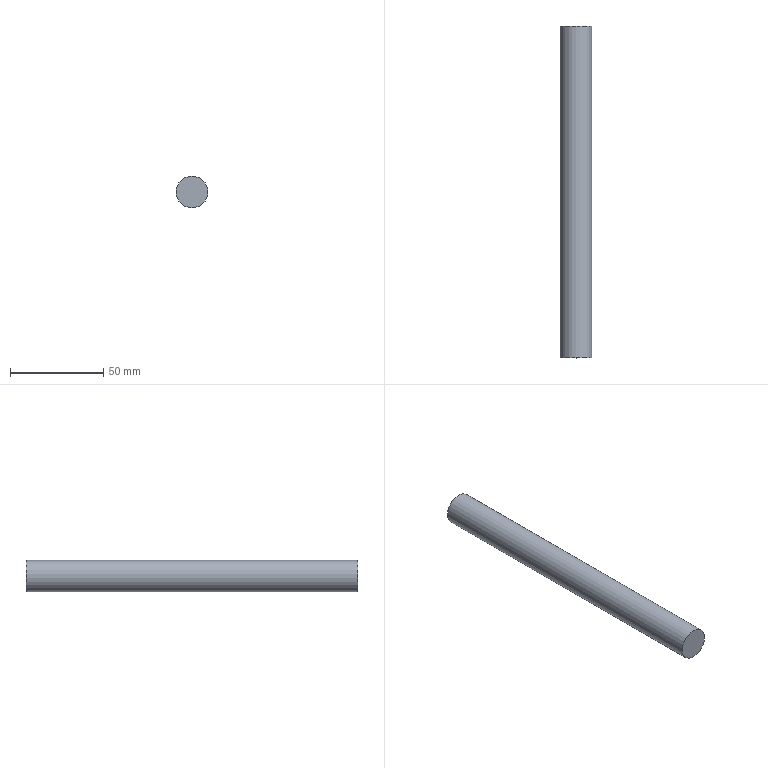Part | NX | features solid 2 | 1 solid | 3 faces | box 17 x 178 x 17 mm | volume 40402 mm3 | plane 2 | cylinder 1 | commonest cylinder face diameters 17 x1
STEP:
#1=CARTESIAN_POINT('',(-296.5,105.,367.5));
#2=VERTEX_POINT('',#1);
#3=CARTESIAN_POINT('',(-296.5,105.,359.));
#4=DIRECTION('',(0.000000011,-1.,0.00000017));
#5=DIRECTION('',(-0.000000001,0.00000017,1.));
#6=AXIS2_PLACEMENT_3D('',#3,#4,#5);
#7=CIRCLE('',#6,8.5);
#8=EDGE_CURVE('',#2,#2,#7,.T.);
#9=ORIENTED_EDGE('',*,*,#8,.T.);
#10=EDGE_LOOP('',(#9));
#11=FACE_BOUND('',#10,.T.);
#12=CARTESIAN_POINT('',(-296.5,-73.,367.5));
#13=VERTEX_POINT('',#12);
#14=CARTESIAN_POINT('',(-296.5,-73.,359.));
#15=DIRECTION('',(0.000000011,-1.,0.00000017));
#16=DIRECTION('',(-0.000000001,0.00000017,1.));
#17=AXIS2_PLACEMENT_3D('',#14,#15,#16);
#18=CIRCLE('',#17,8.5);
#19=EDGE_CURVE('',#13,#13,#18,.T.);
#20=ORIENTED_EDGE('',*,*,#19,.F.);
#21=EDGE_LOOP('',(#20));
#22=FACE_BOUND('',#21,.T.);
#23=CARTESIAN_POINT('',(-296.5,-5.,359.));
#24=DIRECTION('',(0.000000011,-1.,0.00000017));
#25=DIRECTION('',(0.000000001,-0.00000017,-1.));
#26=AXIS2_PLACEMENT_3D('',#23,#24,#25);
#27=CYLINDRICAL_SURFACE('',#26,8.5);
#28=ADVANCED_FACE('',(#11,#22),#27,.T.);
#29=ORIENTED_EDGE('',*,*,#8,.F.);
#30=EDGE_LOOP('',(#29));
#31=FACE_BOUND('',#30,.T.);
#32=CARTESIAN_POINT('',(-296.5,105.,359.));
#33=DIRECTION('',(-0.000000011,1.,-0.00000017));
#34=DIRECTION('',(-0.000000001,0.00000017,1.));
#35=AXIS2_PLACEMENT_3D('',#32,#33,#34);
#36=PLANE('',#35);
#37=ADVANCED_FACE('',(#31),#36,.T.);
#38=ORIENTED_EDGE('',*,*,#19,.T.);
#39=EDGE_LOOP('',(#38));
#40=FACE_BOUND('',#39,.T.);
#41=CARTESIAN_POINT('',(-296.5,-73.,359.));
#42=DIRECTION('',(-0.000000011,1.,-0.00000017));
#43=DIRECTION('',(-0.000000001,0.00000017,1.));
#44=AXIS2_PLACEMENT_3D('',#41,#42,#43);
#45=PLANE('',#44);
#46=ADVANCED_FACE('',(#40),#45,.F.);
#47=CLOSED_SHELL('',(#28,#37,#46));
#48=MANIFOLD_SOLID_BREP('',#47);
#49=(LENGTH_UNIT()NAMED_UNIT(*)SI_UNIT(.MILLI.,.METRE.));
#50=UNCERTAINTY_MEASURE_WITH_UNIT(LENGTH_MEASURE(0.00001),#49,'','');
#51=(NAMED_UNIT(*)PLANE_ANGLE_UNIT()SI_UNIT($,.RADIAN.));
#52=(NAMED_UNIT(*)SI_UNIT($,.STERADIAN.)SOLID_ANGLE_UNIT());
#53=(GEOMETRIC_REPRESENTATION_CONTEXT(3)GLOBAL_UNCERTAINTY_ASSIGNED_CONTEXT((#50))GLOBAL_UNIT_ASSIGNED_CONTEXT((#49,#51,#52))REPRESENTATION_CONTEXT('',''));
#54=ADVANCED_BREP_SHAPE_REPRESENTATION('',(#48),#53);